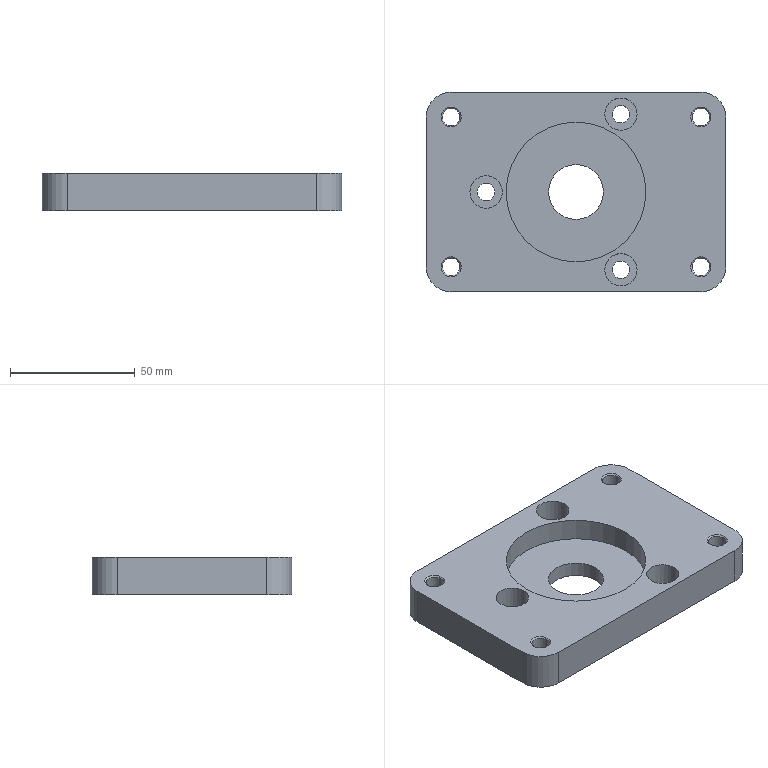Part | STEP file | BCC3 H16_14 | 1 solid | 54 faces | box 120 x 80 x 15 mm | volume 111656 mm3 | cylinder 28 | cone 16 | plane 10 | commonest cylinder face diameters 7 x14 13 x6 20 x4 22 x2 56 x2